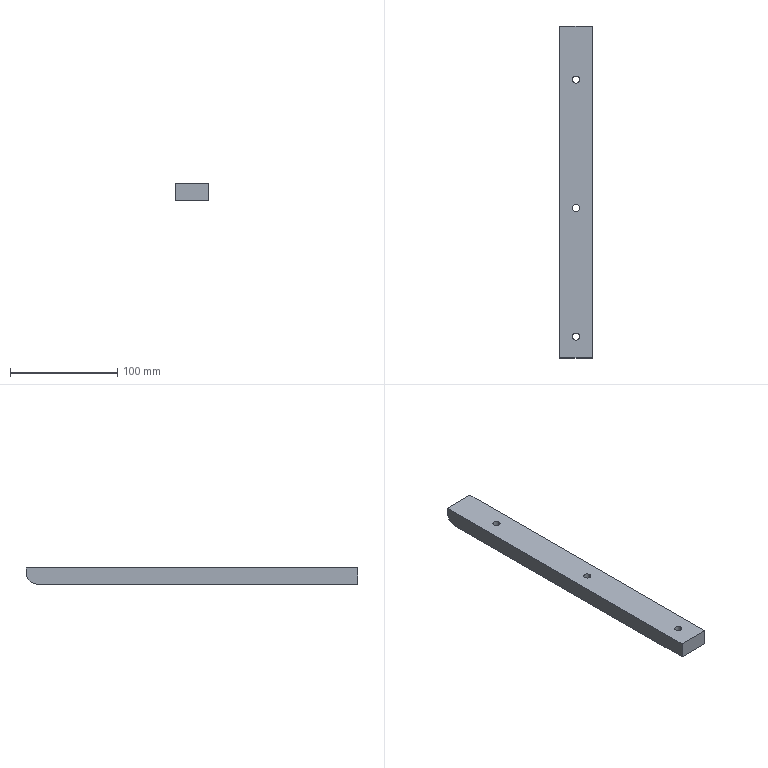Part | SolidWorks | features Extrusion 1, Fillet 1, HoleWzd 1 | 1 solid | 22 faces | box 30 x 310 x 15 mm | volume 136076 mm3 | cylinder 13 | plane 9 | commonest cylinder face diameters 6.6 x6 11 x6 20 x1
STEP:
#1=CARTESIAN_POINT('',(5.5,105.,6.8));
#2=VERTEX_POINT('',#1);
#3=CARTESIAN_POINT('',(-5.5,105.,6.8));
#4=VERTEX_POINT('',#3);
#5=CARTESIAN_POINT('',(0.,105.,6.8));
#6=DIRECTION('',(0.,0.,-1.));
#7=DIRECTION('',(-1.,0.,0.));
#8=AXIS2_PLACEMENT_3D('',#5,#6,#7);
#9=CIRCLE('',#8,5.5);
#10=EDGE_CURVE('',#2,#4,#9,.T.);
#11=ORIENTED_EDGE('',*,*,#10,.F.);
#12=CARTESIAN_POINT('',(5.5,105.,0.));
#13=VERTEX_POINT('',#12);
#14=CARTESIAN_POINT('',(5.5,105.,0.));
#15=DIRECTION('',(0.,0.,-1.));
#16=VECTOR('',#15,1000.);
#17=LINE('',#14,#16);
#18=EDGE_CURVE('',#2,#13,#17,.T.);
#19=ORIENTED_EDGE('',*,*,#18,.T.);
#20=CARTESIAN_POINT('',(-5.5,105.,0.));
#21=VERTEX_POINT('',#20);
#22=CARTESIAN_POINT('',(0.,105.,0.));
#23=DIRECTION('',(0.,0.,-1.));
#24=DIRECTION('',(-1.,0.,0.));
#25=AXIS2_PLACEMENT_3D('',#22,#23,#24);
#26=CIRCLE('',#25,5.5);
#27=EDGE_CURVE('',#13,#21,#26,.T.);
#28=ORIENTED_EDGE('',*,*,#27,.T.);
#29=CARTESIAN_POINT('',(-5.5,105.,0.));
#30=DIRECTION('',(0.,0.,-1.));
#31=VECTOR('',#30,1000.);
#32=LINE('',#29,#31);
#33=EDGE_CURVE('',#4,#21,#32,.T.);
#34=ORIENTED_EDGE('',*,*,#33,.F.);
#35=EDGE_LOOP('',(#11,#19,#28,#34));
#36=FACE_OUTER_BOUND('',#35,.T.);
#37=CARTESIAN_POINT('',(0.,105.,0.));
#38=DIRECTION('',(0.,0.,-1.));
#39=DIRECTION('',(-1.,0.,0.));
#40=AXIS2_PLACEMENT_3D('',#37,#38,#39);
#41=CYLINDRICAL_SURFACE('',#40,5.5);
#42=ADVANCED_FACE('',(#36),#41,.F.);
#43=CARTESIAN_POINT('',(3.3,105.,15.));
#44=VERTEX_POINT('',#43);
#45=CARTESIAN_POINT('',(-3.3,105.,15.));
#46=VERTEX_POINT('',#45);
#47=CARTESIAN_POINT('',(0.,105.,15.));
#48=DIRECTION('',(0.,0.,-1.));
#49=DIRECTION('',(-1.,0.,0.));
#50=AXIS2_PLACEMENT_3D('',#47,#48,#49);
#51=CIRCLE('',#50,3.3);
#52=EDGE_CURVE('',#44,#46,#51,.T.);
#53=ORIENTED_EDGE('',*,*,#52,.F.);
#54=CARTESIAN_POINT('',(3.3,105.,6.8));
#55=VERTEX_POINT('',#54);
#56=CARTESIAN_POINT('',(3.3,105.,0.));
#57=DIRECTION('',(0.,0.,-1.));
#58=VECTOR('',#57,1000.);
#59=LINE('',#56,#58);
#60=EDGE_CURVE('',#44,#55,#59,.T.);
#61=ORIENTED_EDGE('',*,*,#60,.T.);
#62=CARTESIAN_POINT('',(-3.3,105.,6.8));
#63=VERTEX_POINT('',#62);
#64=CARTESIAN_POINT('',(0.,105.,6.8));
#65=DIRECTION('',(0.,0.,-1.));
#66=DIRECTION('',(-1.,0.,0.));
#67=AXIS2_PLACEMENT_3D('',#64,#65,#66);
#68=CIRCLE('',#67,3.3);
#69=EDGE_CURVE('',#55,#63,#68,.T.);
#70=ORIENTED_EDGE('',*,*,#69,.T.);
#71=CARTESIAN_POINT('',(-3.3,105.,0.));
#72=DIRECTION('',(0.,0.,-1.));
#73=VECTOR('',#72,1000.);
#74=LINE('',#71,#73);
#75=EDGE_CURVE('',#46,#63,#74,.T.);
#76=ORIENTED_EDGE('',*,*,#75,.F.);
#77=EDGE_LOOP('',(#53,#61,#70,#76));
#78=FACE_OUTER_BOUND('',#77,.T.);
#79=CARTESIAN_POINT('',(0.,105.,0.));
#80=DIRECTION('',(0.,0.,-1.));
#81=DIRECTION('',(-1.,0.,0.));
#82=AXIS2_PLACEMENT_3D('',#79,#80,#81);
#83=CYLINDRICAL_SURFACE('',#82,3.3);
#84=ADVANCED_FACE('',(#78),#83,.F.);
#85=CARTESIAN_POINT('',(5.5,-15.,6.8));
#86=VERTEX_POINT('',#85);
#87=CARTESIAN_POINT('',(-5.5,-15.,6.8));
#88=VERTEX_POINT('',#87);
#89=CARTESIAN_POINT('',(0.,-15.,6.8));
#90=DIRECTION('',(0.,0.,-1.));
#91=DIRECTION('',(-1.,0.,0.));
#92=AXIS2_PLACEMENT_3D('',#89,#90,#91);
#93=CIRCLE('',#92,5.5);
#94=EDGE_CURVE('',#86,#88,#93,.T.);
#95=ORIENTED_EDGE('',*,*,#94,.F.);
#96=CARTESIAN_POINT('',(5.5,-15.,0.));
#97=VERTEX_POINT('',#96);
#98=CARTESIAN_POINT('',(5.5,-15.,0.));
#99=DIRECTION('',(0.,0.,-1.));
#100=VECTOR('',#99,1000.);
#101=LINE('',#98,#100);
#102=EDGE_CURVE('',#86,#97,#101,.T.);
#103=ORIENTED_EDGE('',*,*,#102,.T.);
#104=CARTESIAN_POINT('',(-5.5,-15.,0.));
#105=VERTEX_POINT('',#104);
#106=CARTESIAN_POINT('',(0.,-15.,0.));
#107=DIRECTION('',(0.,0.,-1.));
#108=DIRECTION('',(-1.,0.,0.));
#109=AXIS2_PLACEMENT_3D('',#106,#107,#108);
#110=CIRCLE('',#109,5.5);
#111=EDGE_CURVE('',#97,#105,#110,.T.);
#112=ORIENTED_EDGE('',*,*,#111,.T.);
#113=CARTESIAN_POINT('',(-5.5,-15.,0.));
#114=DIRECTION('',(0.,0.,-1.));
#115=VECTOR('',#114,1000.);
#116=LINE('',#113,#115);
#117=EDGE_CURVE('',#88,#105,#116,.T.);
#118=ORIENTED_EDGE('',*,*,#117,.F.);
#119=EDGE_LOOP('',(#95,#103,#112,#118));
#120=FACE_OUTER_BOUND('',#119,.T.);
#121=CARTESIAN_POINT('',(0.,-15.,0.));
#122=DIRECTION('',(0.,0.,-1.));
#123=DIRECTION('',(-1.,0.,0.));
#124=AXIS2_PLACEMENT_3D('',#121,#122,#123);
#125=CYLINDRICAL_SURFACE('',#124,5.5);
#126=ADVANCED_FACE('',(#120),#125,.F.);
#127=CARTESIAN_POINT('',(3.3,-15.,15.));
#128=VERTEX_POINT('',#127);
#129=CARTESIAN_POINT('',(-3.3,-15.,15.));
#130=VERTEX_POINT('',#129);
#131=CARTESIAN_POINT('',(0.,-15.,15.));
#132=DIRECTION('',(0.,0.,-1.));
#133=DIRECTION('',(-1.,0.,0.));
#134=AXIS2_PLACEMENT_3D('',#131,#132,#133);
#135=CIRCLE('',#134,3.3);
#136=EDGE_CURVE('',#128,#130,#135,.T.);
#137=ORIENTED_EDGE('',*,*,#136,.F.);
#138=CARTESIAN_POINT('',(3.3,-15.,6.8));
#139=VERTEX_POINT('',#138);
#140=CARTESIAN_POINT('',(3.3,-15.,0.));
#141=DIRECTION('',(0.,0.,-1.));
#142=VECTOR('',#141,1000.);
#143=LINE('',#140,#142);
#144=EDGE_CURVE('',#128,#139,#143,.T.);
#145=ORIENTED_EDGE('',*,*,#144,.T.);
#146=CARTESIAN_POINT('',(-3.3,-15.,6.8));
#147=VERTEX_POINT('',#146);
#148=CARTESIAN_POINT('',(0.,-15.,6.8));
#149=DIRECTION('',(0.,0.,-1.));
#150=DIRECTION('',(-1.,0.,0.));
#151=AXIS2_PLACEMENT_3D('',#148,#149,#150);
#152=CIRCLE('',#151,3.3);
#153=EDGE_CURVE('',#139,#147,#152,.T.);
#154=ORIENTED_EDGE('',*,*,#153,.T.);
#155=CARTESIAN_POINT('',(-3.3,-15.,0.));
#156=DIRECTION('',(0.,0.,-1.));
#157=VECTOR('',#156,1000.);
#158=LINE('',#155,#157);
#159=EDGE_CURVE('',#130,#147,#158,.T.);
#160=ORIENTED_EDGE('',*,*,#159,.F.);
#161=EDGE_LOOP('',(#137,#145,#154,#160));
#162=FACE_OUTER_BOUND('',#161,.T.);
#163=CARTESIAN_POINT('',(0.,-15.,0.));
#164=DIRECTION('',(0.,0.,-1.));
#165=DIRECTION('',(-1.,0.,0.));
#166=AXIS2_PLACEMENT_3D('',#163,#164,#165);
#167=CYLINDRICAL_SURFACE('',#166,3.3);
#168=ADVANCED_FACE('',(#162),#167,.F.);
#169=CARTESIAN_POINT('',(5.5,-135.,6.8));
#170=VERTEX_POINT('',#169);
#171=CARTESIAN_POINT('',(-5.5,-135.,6.8));
#172=VERTEX_POINT('',#171);
#173=CARTESIAN_POINT('',(0.,-135.,6.8));
#174=DIRECTION('',(0.,0.,-1.));
#175=DIRECTION('',(-1.,0.,0.));
#176=AXIS2_PLACEMENT_3D('',#173,#174,#175);
#177=CIRCLE('',#176,5.5);
#178=EDGE_CURVE('',#170,#172,#177,.T.);
#179=ORIENTED_EDGE('',*,*,#178,.F.);
#180=CARTESIAN_POINT('',(5.5,-135.,0.));
#181=VERTEX_POINT('',#180);
#182=CARTESIAN_POINT('',(5.5,-135.,0.));
#183=DIRECTION('',(0.,0.,-1.));
#184=VECTOR('',#183,1000.);
#185=LINE('',#182,#184);
#186=EDGE_CURVE('',#170,#181,#185,.T.);
#187=ORIENTED_EDGE('',*,*,#186,.T.);
#188=CARTESIAN_POINT('',(-5.5,-135.,0.));
#189=VERTEX_POINT('',#188);
#190=CARTESIAN_POINT('',(0.,-135.,0.));
#191=DIRECTION('',(0.,0.,-1.));
#192=DIRECTION('',(-1.,0.,0.));
#193=AXIS2_PLACEMENT_3D('',#190,#191,#192);
#194=CIRCLE('',#193,5.5);
#195=EDGE_CURVE('',#181,#189,#194,.T.);
#196=ORIENTED_EDGE('',*,*,#195,.T.);
#197=CARTESIAN_POINT('',(-5.5,-135.,0.));
#198=DIRECTION('',(0.,0.,-1.));
#199=VECTOR('',#198,1000.);
#200=LINE('',#197,#199);
#201=EDGE_CURVE('',#172,#189,#200,.T.);
#202=ORIENTED_EDGE('',*,*,#201,.F.);
#203=EDGE_LOOP('',(#179,#187,#196,#202));
#204=FACE_OUTER_BOUND('',#203,.T.);
#205=CARTESIAN_POINT('',(0.,-135.,0.));
#206=DIRECTION('',(0.,0.,-1.));
#207=DIRECTION('',(-1.,0.,0.));
#208=AXIS2_PLACEMENT_3D('',#205,#206,#207);
#209=CYLINDRICAL_SURFACE('',#208,5.5);
#210=ADVANCED_FACE('',(#204),#209,.F.);
#211=CARTESIAN_POINT('',(3.3,-135.,15.));
#212=VERTEX_POINT('',#211);
#213=CARTESIAN_POINT('',(-3.3,-135.,15.));
#214=VERTEX_POINT('',#213);
#215=CARTESIAN_POINT('',(0.,-135.,15.));
#216=DIRECTION('',(0.,0.,-1.));
#217=DIRECTION('',(-1.,0.,0.));
#218=AXIS2_PLACEMENT_3D('',#215,#216,#217);
#219=CIRCLE('',#218,3.3);
#220=EDGE_CURVE('',#212,#214,#219,.T.);
#221=ORIENTED_EDGE('',*,*,#220,.F.);
#222=CARTESIAN_POINT('',(3.3,-135.,6.8));
#223=VERTEX_POINT('',#222);
#224=CARTESIAN_POINT('',(3.3,-135.,0.));
#225=DIRECTION('',(0.,0.,-1.));
#226=VECTOR('',#225,1000.);
#227=LINE('',#224,#226);
#228=EDGE_CURVE('',#212,#223,#227,.T.);
#229=ORIENTED_EDGE('',*,*,#228,.T.);
#230=CARTESIAN_POINT('',(-3.3,-135.,6.8));
#231=VERTEX_POINT('',#230);
#232=CARTESIAN_POINT('',(0.,-135.,6.8));
#233=DIRECTION('',(0.,0.,-1.));
#234=DIRECTION('',(-1.,0.,0.));
#235=AXIS2_PLACEMENT_3D('',#232,#233,#234);
#236=CIRCLE('',#235,3.3);
#237=EDGE_CURVE('',#223,#231,#236,.T.);
#238=ORIENTED_EDGE('',*,*,#237,.T.);
#239=CARTESIAN_POINT('',(-3.3,-135.,0.));
#240=DIRECTION('',(0.,0.,-1.));
#241=VECTOR('',#240,1000.);
#242=LINE('',#239,#241);
#243=EDGE_CURVE('',#214,#231,#242,.T.);
#244=ORIENTED_EDGE('',*,*,#243,.F.);
#245=EDGE_LOOP('',(#221,#229,#238,#244));
#246=FACE_OUTER_BOUND('',#245,.T.);
#247=CARTESIAN_POINT('',(0.,-135.,0.));
#248=DIRECTION('',(0.,0.,-1.));
#249=DIRECTION('',(-1.,0.,0.));
#250=AXIS2_PLACEMENT_3D('',#247,#248,#249);
#251=CYLINDRICAL_SURFACE('',#250,3.3);
#252=ADVANCED_FACE('',(#246),#251,.F.);
#253=CARTESIAN_POINT('',(15.,-155.,0.));
#254=VERTEX_POINT('',#253);
#255=CARTESIAN_POINT('',(15.,145.,0.));
#256=VERTEX_POINT('',#255);
#257=CARTESIAN_POINT('',(15.,155.,0.));
#258=DIRECTION('',(0.,1.,0.));
#259=VECTOR('',#258,1000.);
#260=LINE('',#257,#259);
#261=EDGE_CURVE('',#254,#256,#260,.T.);
#262=ORIENTED_EDGE('',*,*,#261,.T.);
#263=CARTESIAN_POINT('',(15.,155.,10.));
#264=VERTEX_POINT('',#263);
#265=CARTESIAN_POINT('',(15.,145.,10.));
#266=DIRECTION('',(1.,0.,0.));
#267=DIRECTION('',(0.,-1.,0.));
#268=AXIS2_PLACEMENT_3D('',#265,#266,#267);
#269=CIRCLE('',#268,10.);
#270=EDGE_CURVE('',#256,#264,#269,.T.);
#271=ORIENTED_EDGE('',*,*,#270,.T.);
#272=CARTESIAN_POINT('',(15.,155.,15.));
#273=VERTEX_POINT('',#272);
#274=CARTESIAN_POINT('',(15.,155.,15.));
#275=DIRECTION('',(0.,0.,-1.));
#276=VECTOR('',#275,1000.);
#277=LINE('',#274,#276);
#278=EDGE_CURVE('',#273,#264,#277,.T.);
#279=ORIENTED_EDGE('',*,*,#278,.F.);
#280=CARTESIAN_POINT('',(15.,-155.,15.));
#281=VERTEX_POINT('',#280);
#282=CARTESIAN_POINT('',(15.,155.,15.));
#283=DIRECTION('',(0.,1.,0.));
#284=VECTOR('',#283,1000.);
#285=LINE('',#282,#284);
#286=EDGE_CURVE('',#281,#273,#285,.T.);
#287=ORIENTED_EDGE('',*,*,#286,.F.);
#288=CARTESIAN_POINT('',(15.,-155.,15.));
#289=DIRECTION('',(0.,0.,-1.));
#290=VECTOR('',#289,1000.);
#291=LINE('',#288,#290);
#292=EDGE_CURVE('',#281,#254,#291,.T.);
#293=ORIENTED_EDGE('',*,*,#292,.T.);
#294=EDGE_LOOP('',(#262,#271,#279,#287,#293));
#295=FACE_OUTER_BOUND('',#294,.T.);
#296=CARTESIAN_POINT('',(15.,155.,15.));
#297=DIRECTION('',(-1.,0.,0.));
#298=DIRECTION('',(0.,-1.,0.));
#299=AXIS2_PLACEMENT_3D('',#296,#297,#298);
#300=PLANE('',#299);
#301=ADVANCED_FACE('',(#295),#300,.F.);
#302=ORIENTED_EDGE('',*,*,#278,.T.);
#303=CARTESIAN_POINT('',(-15.,155.,10.));
#304=VERTEX_POINT('',#303);
#305=CARTESIAN_POINT('',(-15.,155.,10.));
#306=DIRECTION('',(-1.,0.,0.));
#307=VECTOR('',#306,1000.);
#308=LINE('',#305,#307);
#309=EDGE_CURVE('',#264,#304,#308,.T.);
#310=ORIENTED_EDGE('',*,*,#309,.T.);
#311=CARTESIAN_POINT('',(-15.,155.,15.));
#312=VERTEX_POINT('',#311);
#313=CARTESIAN_POINT('',(-15.,155.,15.));
#314=DIRECTION('',(0.,0.,-1.));
#315=VECTOR('',#314,1000.);
#316=LINE('',#313,#315);
#317=EDGE_CURVE('',#312,#304,#316,.T.);
#318=ORIENTED_EDGE('',*,*,#317,.F.);
#319=CARTESIAN_POINT('',(-15.,155.,15.));
#320=DIRECTION('',(-1.,0.,0.));
#321=VECTOR('',#320,1000.);
#322=LINE('',#319,#321);
#323=EDGE_CURVE('',#273,#312,#322,.T.);
#324=ORIENTED_EDGE('',*,*,#323,.F.);
#325=EDGE_LOOP('',(#302,#310,#318,#324));
#326=FACE_OUTER_BOUND('',#325,.T.);
#327=CARTESIAN_POINT('',(-15.,155.,15.));
#328=DIRECTION('',(0.,-1.,0.));
#329=DIRECTION('',(0.,0.,-1.));
#330=AXIS2_PLACEMENT_3D('',#327,#328,#329);
#331=PLANE('',#330);
#332=ADVANCED_FACE('',(#326),#331,.F.);
#333=ORIENTED_EDGE('',*,*,#317,.T.);
#334=CARTESIAN_POINT('',(-15.,145.,0.));
#335=VERTEX_POINT('',#334);
#336=CARTESIAN_POINT('',(-15.,145.,10.));
#337=DIRECTION('',(-1.,0.,0.));
#338=DIRECTION('',(0.,1.,0.));
#339=AXIS2_PLACEMENT_3D('',#336,#337,#338);
#340=CIRCLE('',#339,10.);
#341=EDGE_CURVE('',#304,#335,#340,.T.);
#342=ORIENTED_EDGE('',*,*,#341,.T.);
#343=CARTESIAN_POINT('',(-15.,-155.,0.));
#344=VERTEX_POINT('',#343);
#345=CARTESIAN_POINT('',(-15.,155.,0.));
#346=DIRECTION('',(0.,-1.,0.));
#347=VECTOR('',#346,1000.);
#348=LINE('',#345,#347);
#349=EDGE_CURVE('',#335,#344,#348,.T.);
#350=ORIENTED_EDGE('',*,*,#349,.T.);
#351=CARTESIAN_POINT('',(-15.,-155.,15.));
#352=VERTEX_POINT('',#351);
#353=CARTESIAN_POINT('',(-15.,-155.,15.));
#354=DIRECTION('',(0.,0.,-1.));
#355=VECTOR('',#354,1000.);
#356=LINE('',#353,#355);
#357=EDGE_CURVE('',#352,#344,#356,.T.);
#358=ORIENTED_EDGE('',*,*,#357,.F.);
#359=CARTESIAN_POINT('',(-15.,155.,15.));
#360=DIRECTION('',(0.,-1.,0.));
#361=VECTOR('',#360,1000.);
#362=LINE('',#359,#361);
#363=EDGE_CURVE('',#312,#352,#362,.T.);
#364=ORIENTED_EDGE('',*,*,#363,.F.);
#365=EDGE_LOOP('',(#333,#342,#350,#358,#364));
#366=FACE_OUTER_BOUND('',#365,.T.);
#367=CARTESIAN_POINT('',(-15.,155.,15.));
#368=DIRECTION('',(1.,0.,0.));
#369=DIRECTION('',(0.,1.,0.));
#370=AXIS2_PLACEMENT_3D('',#367,#368,#369);
#371=PLANE('',#370);
#372=ADVANCED_FACE('',(#366),#371,.F.);
#373=CARTESIAN_POINT('',(-15.,-155.,0.));
#374=DIRECTION('',(1.,0.,0.));
#375=VECTOR('',#374,1000.);
#376=LINE('',#373,#375);
#377=EDGE_CURVE('',#344,#254,#376,.T.);
#378=ORIENTED_EDGE('',*,*,#377,.T.);
#379=ORIENTED_EDGE('',*,*,#292,.F.);
#380=CARTESIAN_POINT('',(-15.,-155.,15.));
#381=DIRECTION('',(1.,0.,0.));
#382=VECTOR('',#381,1000.);
#383=LINE('',#380,#382);
#384=EDGE_CURVE('',#352,#281,#383,.T.);
#385=ORIENTED_EDGE('',*,*,#384,.F.);
#386=ORIENTED_EDGE('',*,*,#357,.T.);
#387=EDGE_LOOP('',(#378,#379,#385,#386));
#388=FACE_OUTER_BOUND('',#387,.T.);
#389=CARTESIAN_POINT('',(-15.,-155.,15.));
#390=DIRECTION('',(0.,1.,0.));
#391=DIRECTION('',(0.,0.,1.));
#392=AXIS2_PLACEMENT_3D('',#389,#390,#391);
#393=PLANE('',#392);
#394=ADVANCED_FACE('',(#388),#393,.F.);
#395=CARTESIAN_POINT('',(0.,105.,15.));
#396=DIRECTION('',(0.,0.,-1.));
#397=DIRECTION('',(-1.,0.,0.));
#398=AXIS2_PLACEMENT_3D('',#395,#396,#397);
#399=CIRCLE('',#398,3.3);
#400=EDGE_CURVE('',#46,#44,#399,.T.);
#401=ORIENTED_EDGE('',*,*,#400,.T.);
#402=ORIENTED_EDGE('',*,*,#52,.T.);
#403=EDGE_LOOP('',(#401,#402));
#404=FACE_BOUND('',#403,.T.);
#405=CARTESIAN_POINT('',(0.,-15.,15.));
#406=DIRECTION('',(0.,0.,-1.));
#407=DIRECTION('',(-1.,0.,0.));
#408=AXIS2_PLACEMENT_3D('',#405,#406,#407);
#409=CIRCLE('',#408,3.3);
#410=EDGE_CURVE('',#130,#128,#409,.T.);
#411=ORIENTED_EDGE('',*,*,#410,.T.);
#412=ORIENTED_EDGE('',*,*,#136,.T.);
#413=EDGE_LOOP('',(#411,#412));
#414=FACE_BOUND('',#413,.T.);
#415=CARTESIAN_POINT('',(0.,-135.,15.));
#416=DIRECTION('',(0.,0.,-1.));
#417=DIRECTION('',(-1.,0.,0.));
#418=AXIS2_PLACEMENT_3D('',#415,#416,#417);
#419=CIRCLE('',#418,3.3);
#420=EDGE_CURVE('',#214,#212,#419,.T.);
#421=ORIENTED_EDGE('',*,*,#420,.T.);
#422=ORIENTED_EDGE('',*,*,#220,.T.);
#423=EDGE_LOOP('',(#421,#422));
#424=FACE_BOUND('',#423,.T.);
#425=ORIENTED_EDGE('',*,*,#286,.T.);
#426=ORIENTED_EDGE('',*,*,#323,.T.);
#427=ORIENTED_EDGE('',*,*,#363,.T.);
#428=ORIENTED_EDGE('',*,*,#384,.T.);
#429=EDGE_LOOP('',(#425,#426,#427,#428));
#430=FACE_OUTER_BOUND('',#429,.T.);
#431=CARTESIAN_POINT('',(0.,0.,15.));
#432=DIRECTION('',(0.,0.,1.));
#433=DIRECTION('',(1.,0.,0.));
#434=AXIS2_PLACEMENT_3D('',#431,#432,#433);
#435=PLANE('',#434);
#436=ADVANCED_FACE('',(#404,#414,#424,#430),#435,.T.);
#437=CARTESIAN_POINT('',(0.,105.,0.));
#438=DIRECTION('',(0.,0.,-1.));
#439=DIRECTION('',(-1.,0.,0.));
#440=AXIS2_PLACEMENT_3D('',#437,#438,#439);
#441=CIRCLE('',#440,5.5);
#442=EDGE_CURVE('',#21,#13,#441,.T.);
#443=ORIENTED_EDGE('',*,*,#442,.F.);
#444=ORIENTED_EDGE('',*,*,#27,.F.);
#445=EDGE_LOOP('',(#443,#444));
#446=FACE_BOUND('',#445,.T.);
#447=CARTESIAN_POINT('',(0.,-15.,0.));
#448=DIRECTION('',(0.,0.,-1.));
#449=DIRECTION('',(-1.,0.,0.));
#450=AXIS2_PLACEMENT_3D('',#447,#448,#449);
#451=CIRCLE('',#450,5.5);
#452=EDGE_CURVE('',#105,#97,#451,.T.);
#453=ORIENTED_EDGE('',*,*,#452,.F.);
#454=ORIENTED_EDGE('',*,*,#111,.F.);
#455=EDGE_LOOP('',(#453,#454));
#456=FACE_BOUND('',#455,.T.);
#457=CARTESIAN_POINT('',(0.,-135.,0.));
#458=DIRECTION('',(0.,0.,-1.));
#459=DIRECTION('',(-1.,0.,0.));
#460=AXIS2_PLACEMENT_3D('',#457,#458,#459);
#461=CIRCLE('',#460,5.5);
#462=EDGE_CURVE('',#189,#181,#461,.T.);
#463=ORIENTED_EDGE('',*,*,#462,.F.);
#464=ORIENTED_EDGE('',*,*,#195,.F.);
#465=EDGE_LOOP('',(#463,#464));
#466=FACE_BOUND('',#465,.T.);
#467=ORIENTED_EDGE('',*,*,#349,.F.);
#468=CARTESIAN_POINT('',(0.,145.,0.));
#469=DIRECTION('',(1.,0.,0.));
#470=VECTOR('',#469,1000.);
#471=LINE('',#468,#470);
#472=EDGE_CURVE('',#335,#256,#471,.T.);
#473=ORIENTED_EDGE('',*,*,#472,.T.);
#474=ORIENTED_EDGE('',*,*,#261,.F.);
#475=ORIENTED_EDGE('',*,*,#377,.F.);
#476=EDGE_LOOP('',(#467,#473,#474,#475));
#477=FACE_OUTER_BOUND('',#476,.T.);
#478=CARTESIAN_POINT('',(0.,0.,0.));
#479=DIRECTION('',(0.,0.,1.));
#480=DIRECTION('',(1.,0.,0.));
#481=AXIS2_PLACEMENT_3D('',#478,#479,#480);
#482=PLANE('',#481);
#483=ADVANCED_FACE('',(#446,#456,#466,#477),#482,.F.);
#484=ORIENTED_EDGE('',*,*,#228,.F.);
#485=ORIENTED_EDGE('',*,*,#420,.F.);
#486=ORIENTED_EDGE('',*,*,#243,.T.);
#487=CARTESIAN_POINT('',(0.,-135.,6.8));
#488=DIRECTION('',(0.,0.,-1.));
#489=DIRECTION('',(-1.,0.,0.));
#490=AXIS2_PLACEMENT_3D('',#487,#488,#489);
#491=CIRCLE('',#490,3.3);
#492=EDGE_CURVE('',#231,#223,#491,.T.);
#493=ORIENTED_EDGE('',*,*,#492,.T.);
#494=EDGE_LOOP('',(#484,#485,#486,#493));
#495=FACE_OUTER_BOUND('',#494,.T.);
#496=CARTESIAN_POINT('',(0.,-135.,0.));
#497=DIRECTION('',(0.,0.,-1.));
#498=DIRECTION('',(-1.,0.,0.));
#499=AXIS2_PLACEMENT_3D('',#496,#497,#498);
#500=CYLINDRICAL_SURFACE('',#499,3.3);
#501=ADVANCED_FACE('',(#495),#500,.F.);
#502=ORIENTED_EDGE('',*,*,#492,.F.);
#503=ORIENTED_EDGE('',*,*,#237,.F.);
#504=EDGE_LOOP('',(#502,#503));
#505=FACE_BOUND('',#504,.T.);
#506=CARTESIAN_POINT('',(0.,-135.,6.8));
#507=DIRECTION('',(0.,0.,-1.));
#508=DIRECTION('',(-1.,0.,0.));
#509=AXIS2_PLACEMENT_3D('',#506,#507,#508);
#510=CIRCLE('',#509,5.5);
#511=EDGE_CURVE('',#172,#170,#510,.T.);
#512=ORIENTED_EDGE('',*,*,#511,.T.);
#513=ORIENTED_EDGE('',*,*,#178,.T.);
#514=EDGE_LOOP('',(#512,#513));
#515=FACE_OUTER_BOUND('',#514,.T.);
#516=CARTESIAN_POINT('',(3.3,-135.,6.8));
#517=DIRECTION('',(0.,0.,1.));
#518=DIRECTION('',(1.,0.,0.));
#519=AXIS2_PLACEMENT_3D('',#516,#517,#518);
#520=PLANE('',#519);
#521=ADVANCED_FACE('',(#505,#515),#520,.F.);
#522=ORIENTED_EDGE('',*,*,#186,.F.);
#523=ORIENTED_EDGE('',*,*,#511,.F.);
#524=ORIENTED_EDGE('',*,*,#201,.T.);
#525=ORIENTED_EDGE('',*,*,#462,.T.);
#526=EDGE_LOOP('',(#522,#523,#524,#525));
#527=FACE_OUTER_BOUND('',#526,.T.);
#528=CARTESIAN_POINT('',(0.,-135.,0.));
#529=DIRECTION('',(0.,0.,-1.));
#530=DIRECTION('',(-1.,0.,0.));
#531=AXIS2_PLACEMENT_3D('',#528,#529,#530);
#532=CYLINDRICAL_SURFACE('',#531,5.5);
#533=ADVANCED_FACE('',(#527),#532,.F.);
#534=ORIENTED_EDGE('',*,*,#144,.F.);
#535=ORIENTED_EDGE('',*,*,#410,.F.);
#536=ORIENTED_EDGE('',*,*,#159,.T.);
#537=CARTESIAN_POINT('',(0.,-15.,6.8));
#538=DIRECTION('',(0.,0.,-1.));
#539=DIRECTION('',(-1.,0.,0.));
#540=AXIS2_PLACEMENT_3D('',#537,#538,#539);
#541=CIRCLE('',#540,3.3);
#542=EDGE_CURVE('',#147,#139,#541,.T.);
#543=ORIENTED_EDGE('',*,*,#542,.T.);
#544=EDGE_LOOP('',(#534,#535,#536,#543));
#545=FACE_OUTER_BOUND('',#544,.T.);
#546=CARTESIAN_POINT('',(0.,-15.,0.));
#547=DIRECTION('',(0.,0.,-1.));
#548=DIRECTION('',(-1.,0.,0.));
#549=AXIS2_PLACEMENT_3D('',#546,#547,#548);
#550=CYLINDRICAL_SURFACE('',#549,3.3);
#551=ADVANCED_FACE('',(#545),#550,.F.);
#552=ORIENTED_EDGE('',*,*,#542,.F.);
#553=ORIENTED_EDGE('',*,*,#153,.F.);
#554=EDGE_LOOP('',(#552,#553));
#555=FACE_BOUND('',#554,.T.);
#556=CARTESIAN_POINT('',(0.,-15.,6.8));
#557=DIRECTION('',(0.,0.,-1.));
#558=DIRECTION('',(-1.,0.,0.));
#559=AXIS2_PLACEMENT_3D('',#556,#557,#558);
#560=CIRCLE('',#559,5.5);
#561=EDGE_CURVE('',#88,#86,#560,.T.);
#562=ORIENTED_EDGE('',*,*,#561,.T.);
#563=ORIENTED_EDGE('',*,*,#94,.T.);
#564=EDGE_LOOP('',(#562,#563));
#565=FACE_OUTER_BOUND('',#564,.T.);
#566=CARTESIAN_POINT('',(3.3,-15.,6.8));
#567=DIRECTION('',(0.,0.,1.));
#568=DIRECTION('',(1.,0.,0.));
#569=AXIS2_PLACEMENT_3D('',#566,#567,#568);
#570=PLANE('',#569);
#571=ADVANCED_FACE('',(#555,#565),#570,.F.);
#572=ORIENTED_EDGE('',*,*,#102,.F.);
#573=ORIENTED_EDGE('',*,*,#561,.F.);
#574=ORIENTED_EDGE('',*,*,#117,.T.);
#575=ORIENTED_EDGE('',*,*,#452,.T.);
#576=EDGE_LOOP('',(#572,#573,#574,#575));
#577=FACE_OUTER_BOUND('',#576,.T.);
#578=CARTESIAN_POINT('',(0.,-15.,0.));
#579=DIRECTION('',(0.,0.,-1.));
#580=DIRECTION('',(-1.,0.,0.));
#581=AXIS2_PLACEMENT_3D('',#578,#579,#580);
#582=CYLINDRICAL_SURFACE('',#581,5.5);
#583=ADVANCED_FACE('',(#577),#582,.F.);
#584=ORIENTED_EDGE('',*,*,#60,.F.);
#585=ORIENTED_EDGE('',*,*,#400,.F.);
#586=ORIENTED_EDGE('',*,*,#75,.T.);
#587=CARTESIAN_POINT('',(0.,105.,6.8));
#588=DIRECTION('',(0.,0.,-1.));
#589=DIRECTION('',(-1.,0.,0.));
#590=AXIS2_PLACEMENT_3D('',#587,#588,#589);
#591=CIRCLE('',#590,3.3);
#592=EDGE_CURVE('',#63,#55,#591,.T.);
#593=ORIENTED_EDGE('',*,*,#592,.T.);
#594=EDGE_LOOP('',(#584,#585,#586,#593));
#595=FACE_OUTER_BOUND('',#594,.T.);
#596=CARTESIAN_POINT('',(0.,105.,0.));
#597=DIRECTION('',(0.,0.,-1.));
#598=DIRECTION('',(-1.,0.,0.));
#599=AXIS2_PLACEMENT_3D('',#596,#597,#598);
#600=CYLINDRICAL_SURFACE('',#599,3.3);
#601=ADVANCED_FACE('',(#595),#600,.F.);
#602=ORIENTED_EDGE('',*,*,#592,.F.);
#603=ORIENTED_EDGE('',*,*,#69,.F.);
#604=EDGE_LOOP('',(#602,#603));
#605=FACE_BOUND('',#604,.T.);
#606=CARTESIAN_POINT('',(0.,105.,6.8));
#607=DIRECTION('',(0.,0.,-1.));
#608=DIRECTION('',(-1.,0.,0.));
#609=AXIS2_PLACEMENT_3D('',#606,#607,#608);
#610=CIRCLE('',#609,5.5);
#611=EDGE_CURVE('',#4,#2,#610,.T.);
#612=ORIENTED_EDGE('',*,*,#611,.T.);
#613=ORIENTED_EDGE('',*,*,#10,.T.);
#614=EDGE_LOOP('',(#612,#613));
#615=FACE_OUTER_BOUND('',#614,.T.);
#616=CARTESIAN_POINT('',(3.3,105.,6.8));
#617=DIRECTION('',(0.,0.,1.));
#618=DIRECTION('',(1.,0.,0.));
#619=AXIS2_PLACEMENT_3D('',#616,#617,#618);
#620=PLANE('',#619);
#621=ADVANCED_FACE('',(#605,#615),#620,.F.);
#622=ORIENTED_EDGE('',*,*,#18,.F.);
#623=ORIENTED_EDGE('',*,*,#611,.F.);
#624=ORIENTED_EDGE('',*,*,#33,.T.);
#625=ORIENTED_EDGE('',*,*,#442,.T.);
#626=EDGE_LOOP('',(#622,#623,#624,#625));
#627=FACE_OUTER_BOUND('',#626,.T.);
#628=CARTESIAN_POINT('',(0.,105.,0.));
#629=DIRECTION('',(0.,0.,-1.));
#630=DIRECTION('',(-1.,0.,0.));
#631=AXIS2_PLACEMENT_3D('',#628,#629,#630);
#632=CYLINDRICAL_SURFACE('',#631,5.5);
#633=ADVANCED_FACE('',(#627),#632,.F.);
#634=ORIENTED_EDGE('',*,*,#270,.F.);
#635=ORIENTED_EDGE('',*,*,#472,.F.);
#636=ORIENTED_EDGE('',*,*,#341,.F.);
#637=ORIENTED_EDGE('',*,*,#309,.F.);
#638=EDGE_LOOP('',(#634,#635,#636,#637));
#639=FACE_OUTER_BOUND('',#638,.T.);
#640=CARTESIAN_POINT('',(-15.,145.,10.));
#641=DIRECTION('',(-1.,0.,0.));
#642=DIRECTION('',(0.,0.,1.));
#643=AXIS2_PLACEMENT_3D('',#640,#641,#642);
#644=CYLINDRICAL_SURFACE('',#643,10.);
#645=ADVANCED_FACE('',(#639),#644,.T.);
#646=CLOSED_SHELL('',(#42,#84,#126,#168,#210,#252,#301,#332,#372,#394,#436,#483,#501,#521,#533,#551,#571,#583,#601,#621,#633,#645));
#647=MANIFOLD_SOLID_BREP('',#646);
#648=CARTESIAN_POINT('',(0.,0.,0.));
#649=DIRECTION('',(0.,0.,1.));
#650=DIRECTION('',(1.,0.,0.));
#651=AXIS2_PLACEMENT_3D('',#648,#649,#650);
#652=(LENGTH_UNIT()NAMED_UNIT(*)SI_UNIT(.MILLI.,.METRE.));
#653=UNCERTAINTY_MEASURE_WITH_UNIT(LENGTH_MEASURE(0.00001),#652,'','');
#654=(NAMED_UNIT(*)PLANE_ANGLE_UNIT()SI_UNIT($,.RADIAN.));
#655=(NAMED_UNIT(*)SI_UNIT($,.STERADIAN.)SOLID_ANGLE_UNIT());
#656=(GEOMETRIC_REPRESENTATION_CONTEXT(3)GLOBAL_UNCERTAINTY_ASSIGNED_CONTEXT((#653))GLOBAL_UNIT_ASSIGNED_CONTEXT((#652,#654,#655))REPRESENTATION_CONTEXT('',''));
#657=ADVANCED_BREP_SHAPE_REPRESENTATION('',(#647,#651),#656);